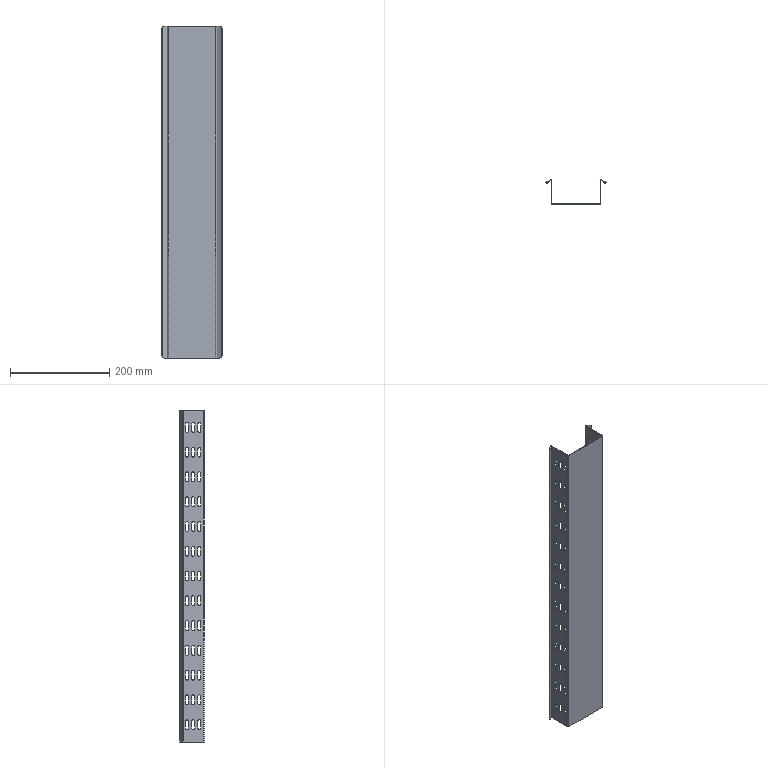Part | SolidWorks | 1 solid | 432 faces | box 121.249 x 49.695 x 670 mm | volume 206402 mm3 | cylinder 246 | plane 186 | commonest cylinder face diameters 6 x234 0.2 x4 3.2 x4 10 x4